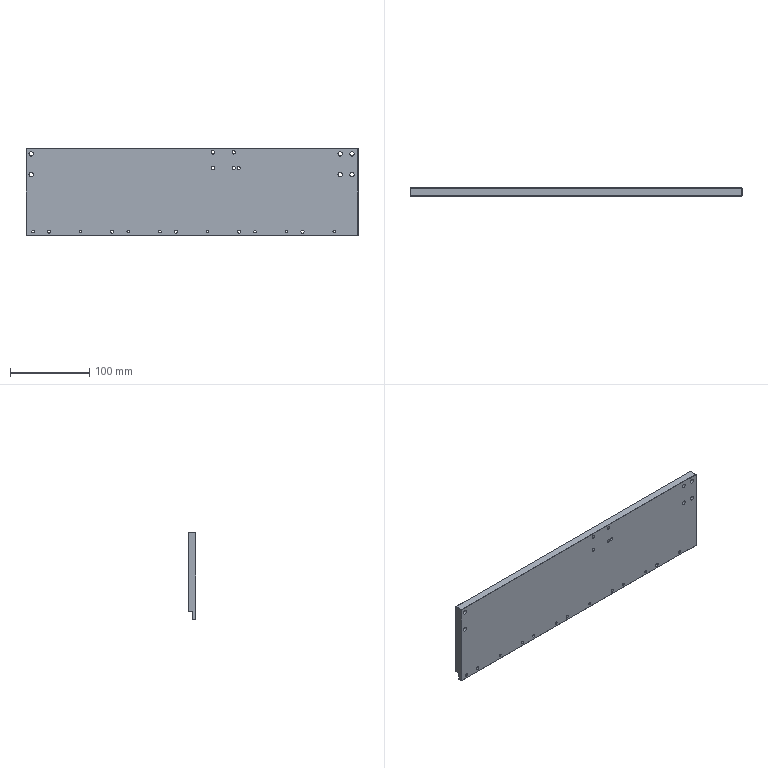Part | NX | 1 solid | 119 faces | box 419 x 10 x 110 mm | volume 434424 mm3 | cone 48 | cylinder 48 | plane 23 | commonest cylinder face diameters 3.3 x16 4 x12 5.5 x12 4.2 x8